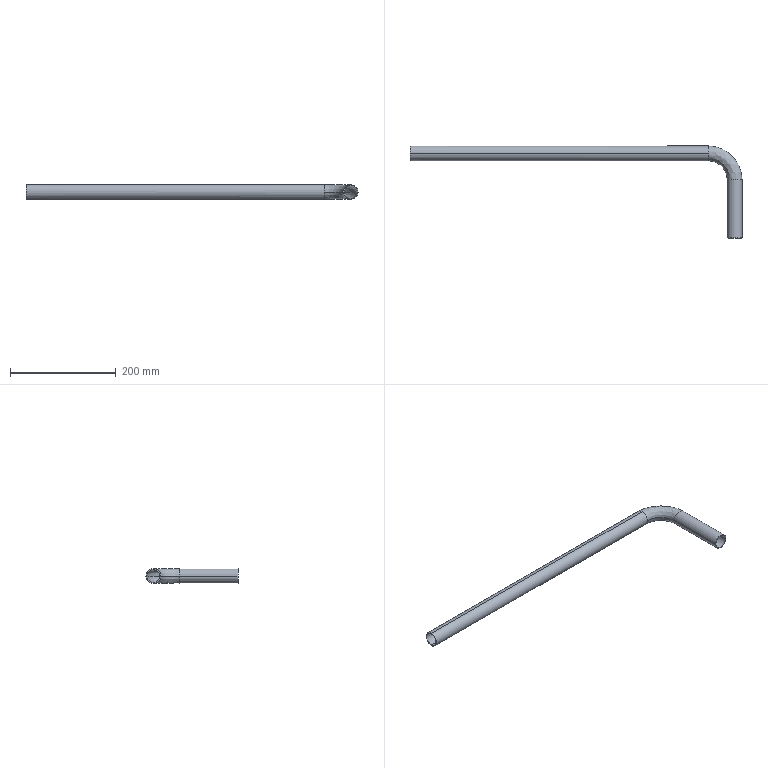Part | STEP file | copper tube 15_default_machined_ | 1 solid | 14 faces | box 627.9 x 174 x 28 mm | volume 93963 mm3 | cylinder 8 | spline 4 | plane 2 | commonest cylinder face diameters 25 x4 28 x4